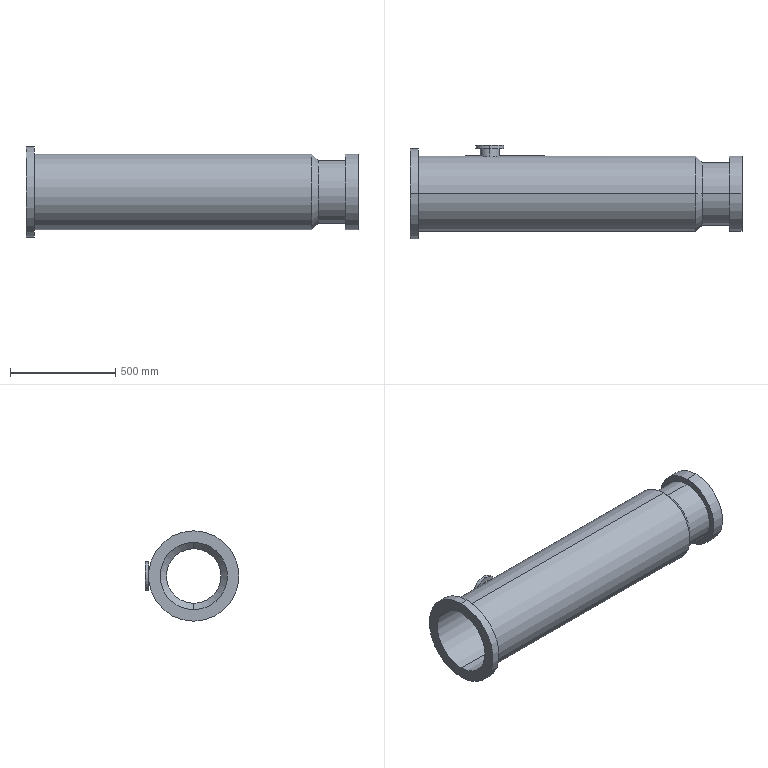Part | SolidWorks | features ICE 4, Revolution 1 | 1 solid | 28 faces | box 1580 x 445 x 430 mm | volume 36909179 mm3 | cylinder 18 | plane 6 | cone 4 | commonest cylinder face diameters 360 x4 80 x2 92 x2 135 x2 260 x2 300 x2
STEP:
#1=CARTESIAN_POINT('',(380.,230.,67.5));
#2=VERTEX_POINT('',#1);
#3=CARTESIAN_POINT('',(380.,230.,-67.5));
#4=VERTEX_POINT('',#3);
#5=CARTESIAN_POINT('',(380.,230.,0.));
#6=DIRECTION('',(0.,1.,0.));
#7=DIRECTION('',(0.,0.,1.));
#8=AXIS2_PLACEMENT_3D('',#5,#6,#7);
#9=CIRCLE('',#8,67.5);
#10=EDGE_CURVE('',#2,#4,#9,.T.);
#11=ORIENTED_EDGE('',*,*,#10,.F.);
#12=CARTESIAN_POINT('',(380.,215.,67.5));
#13=VERTEX_POINT('',#12);
#14=CARTESIAN_POINT('',(380.,230.,67.5));
#15=DIRECTION('',(0.,-1.,0.));
#16=VECTOR('',#15,1000.);
#17=LINE('',#14,#16);
#18=EDGE_CURVE('',#2,#13,#17,.T.);
#19=ORIENTED_EDGE('',*,*,#18,.T.);
#20=CARTESIAN_POINT('',(380.,215.,-67.5));
#21=VERTEX_POINT('',#20);
#22=CARTESIAN_POINT('',(380.,215.,0.));
#23=DIRECTION('',(0.,1.,0.));
#24=DIRECTION('',(0.,0.,1.));
#25=AXIS2_PLACEMENT_3D('',#22,#23,#24);
#26=CIRCLE('',#25,67.5);
#27=EDGE_CURVE('',#13,#21,#26,.T.);
#28=ORIENTED_EDGE('',*,*,#27,.T.);
#29=CARTESIAN_POINT('',(380.,230.,-67.5));
#30=DIRECTION('',(0.,-1.,0.));
#31=VECTOR('',#30,1000.);
#32=LINE('',#29,#31);
#33=EDGE_CURVE('',#4,#21,#32,.T.);
#34=ORIENTED_EDGE('',*,*,#33,.F.);
#35=EDGE_LOOP('',(#11,#19,#28,#34));
#36=FACE_OUTER_BOUND('',#35,.T.);
#37=CARTESIAN_POINT('',(380.,230.,0.));
#38=DIRECTION('',(0.,-1.,0.));
#39=DIRECTION('',(0.,0.,-1.));
#40=AXIS2_PLACEMENT_3D('',#37,#38,#39);
#41=CYLINDRICAL_SURFACE('',#40,67.5);
#42=ADVANCED_FACE('',(#36),#41,.T.);
#43=CARTESIAN_POINT('',(1351.716,0.,-160.));
#44=VERTEX_POINT('',#43);
#45=CARTESIAN_POINT('',(1351.716,0.,160.));
#46=VERTEX_POINT('',#45);
#47=CARTESIAN_POINT('',(1351.716,0.,0.));
#48=DIRECTION('',(-1.,0.,0.));
#49=DIRECTION('',(0.,0.,1.));
#50=AXIS2_PLACEMENT_3D('',#47,#48,#49);
#51=CIRCLE('',#50,160.);
#52=EDGE_CURVE('',#44,#46,#51,.T.);
#53=ORIENTED_EDGE('',*,*,#52,.F.);
#54=CARTESIAN_POINT('',(0.,0.,-160.));
#55=VERTEX_POINT('',#54);
#56=CARTESIAN_POINT('',(0.,0.,-160.));
#57=DIRECTION('',(-1.,0.,0.));
#58=VECTOR('',#57,1000.);
#59=LINE('',#56,#58);
#60=EDGE_CURVE('',#44,#55,#59,.T.);
#61=ORIENTED_EDGE('',*,*,#60,.T.);
#62=CARTESIAN_POINT('',(0.,0.,160.));
#63=VERTEX_POINT('',#62);
#64=CARTESIAN_POINT('',(0.,0.,0.));
#65=DIRECTION('',(-1.,0.,0.));
#66=DIRECTION('',(0.,0.,1.));
#67=AXIS2_PLACEMENT_3D('',#64,#65,#66);
#68=CIRCLE('',#67,160.);
#69=EDGE_CURVE('',#55,#63,#68,.T.);
#70=ORIENTED_EDGE('',*,*,#69,.T.);
#71=CARTESIAN_POINT('',(0.,0.,160.));
#72=DIRECTION('',(-1.,0.,0.));
#73=VECTOR('',#72,1000.);
#74=LINE('',#71,#73);
#75=EDGE_CURVE('',#46,#63,#74,.T.);
#76=ORIENTED_EDGE('',*,*,#75,.F.);
#77=EDGE_LOOP('',(#53,#61,#70,#76));
#78=FACE_OUTER_BOUND('',#77,.T.);
#79=CARTESIAN_POINT('',(0.,0.,0.));
#80=DIRECTION('',(-1.,0.,0.));
#81=DIRECTION('',(0.,0.,1.));
#82=AXIS2_PLACEMENT_3D('',#79,#80,#81);
#83=CYLINDRICAL_SURFACE('',#82,160.);
#84=ADVANCED_FACE('',(#78),#83,.F.);
#85=CARTESIAN_POINT('',(380.,230.,-40.));
#86=VERTEX_POINT('',#85);
#87=CARTESIAN_POINT('',(380.,230.,40.));
#88=VERTEX_POINT('',#87);
#89=CARTESIAN_POINT('',(380.,230.,0.));
#90=DIRECTION('',(0.,1.,0.));
#91=DIRECTION('',(0.,0.,1.));
#92=AXIS2_PLACEMENT_3D('',#89,#90,#91);
#93=CIRCLE('',#92,40.);
#94=EDGE_CURVE('',#86,#88,#93,.T.);
#95=ORIENTED_EDGE('',*,*,#94,.T.);
#96=CARTESIAN_POINT('',(380.,154.919,40.));
#97=VERTEX_POINT('',#96);
#98=CARTESIAN_POINT('',(380.,215.,40.));
#99=DIRECTION('',(0.,-1.,0.));
#100=VECTOR('',#99,1000.);
#101=LINE('',#98,#100);
#102=EDGE_CURVE('',#88,#97,#101,.T.);
#103=ORIENTED_EDGE('',*,*,#102,.T.);
#104=CARTESIAN_POINT('',(380.,154.919,-40.));
#105=VERTEX_POINT('',#104);
#106=CARTESIAN_POINT('',(380.,154.919,-40.));
#107=CARTESIAN_POINT('',(377.384,154.919,-40.));
#108=CARTESIAN_POINT('',(374.776,154.986,-39.746));
#109=CARTESIAN_POINT('',(369.578,155.248,-38.709));
#110=CARTESIAN_POINT('',(367.077,155.439,-37.945));
#111=CARTESIAN_POINT('',(363.464,155.795,-36.445));
#112=CARTESIAN_POINT('',(362.283,155.925,-35.886));
#113=CARTESIAN_POINT('',(360.547,156.135,-34.957));
#114=CARTESIAN_POINT('',(359.973,156.207,-34.632));
#115=CARTESIAN_POINT('',(358.846,156.356,-33.955));
#116=CARTESIAN_POINT('',(358.293,156.432,-33.604));
#117=CARTESIAN_POINT('',(355.581,156.817,-31.789));
#118=CARTESIAN_POINT('',(353.574,157.147,-30.141));
#119=CARTESIAN_POINT('',(351.268,157.561,-27.837));
#120=CARTESIAN_POINT('',(350.817,157.643,-27.364));
#121=CARTESIAN_POINT('',(349.936,157.809,-26.392));
#122=CARTESIAN_POINT('',(349.505,157.892,-25.894));
#123=CARTESIAN_POINT('',(348.257,158.136,-24.375));
#124=CARTESIAN_POINT('',(347.481,158.294,-23.328));
#125=CARTESIAN_POINT('',(345.312,158.749,-20.088));
#126=CARTESIAN_POINT('',(344.079,159.026,-17.795));
#127=CARTESIAN_POINT('',(342.814,159.32,-14.753));
#128=CARTESIAN_POINT('',(342.575,159.376,-14.136));
#129=CARTESIAN_POINT('',(342.131,159.48,-12.898));
#130=CARTESIAN_POINT('',(341.924,159.53,-12.275));
#131=CARTESIAN_POINT('',(341.353,159.667,-10.397));
#132=CARTESIAN_POINT('',(341.034,159.744,-9.131));
#133=CARTESIAN_POINT('',(340.522,159.87,-6.571));
#134=CARTESIAN_POINT('',(340.328,159.918,-5.277));
#135=CARTESIAN_POINT('',(340.132,159.967,-3.315));
#136=CARTESIAN_POINT('',(340.083,159.979,-2.658));
#137=CARTESIAN_POINT('',(340.017,159.996,-1.335));
#138=CARTESIAN_POINT('',(340.,160.,-0.6716));
#139=CARTESIAN_POINT('',(339.999,160.,2.626));
#140=CARTESIAN_POINT('',(340.257,159.935,5.229));
#141=CARTESIAN_POINT('',(341.023,159.747,9.083));
#142=CARTESIAN_POINT('',(341.342,159.669,10.36));
#143=CARTESIAN_POINT('',(342.111,159.485,12.891));
#144=CARTESIAN_POINT('',(342.555,159.38,14.127));
#145=CARTESIAN_POINT('',(344.057,159.031,17.745));
#146=CARTESIAN_POINT('',(345.284,158.755,20.042));
#147=CARTESIAN_POINT('',(347.106,158.373,22.768));
#148=CARTESIAN_POINT('',(347.486,158.294,23.308));
#149=CARTESIAN_POINT('',(348.268,158.135,24.362));
#150=CARTESIAN_POINT('',(348.671,158.055,24.878));
#151=CARTESIAN_POINT('',(349.912,157.812,26.39));
#152=CARTESIAN_POINT('',(350.785,157.647,27.352));
#153=CARTESIAN_POINT('',(352.619,157.318,29.189));
#154=CARTESIAN_POINT('',(353.581,157.153,30.062));
#155=CARTESIAN_POINT('',(355.092,156.908,31.305));
#156=CARTESIAN_POINT('',(355.607,156.827,31.708));
#157=CARTESIAN_POINT('',(356.66,156.667,32.491));
#158=CARTESIAN_POINT('',(357.198,156.587,32.871));
#159=CARTESIAN_POINT('',(359.922,156.2,34.695));
#160=CARTESIAN_POINT('',(362.216,155.918,35.924));
#161=CARTESIAN_POINT('',(365.826,155.562,37.427));
#162=CARTESIAN_POINT('',(367.058,155.454,37.871));
#163=CARTESIAN_POINT('',(368.95,155.312,38.449));
#164=CARTESIAN_POINT('',(369.589,155.267,38.627));
#165=CARTESIAN_POINT('',(370.868,155.187,38.949));
#166=CARTESIAN_POINT('',(371.51,155.15,39.094));
#167=CARTESIAN_POINT('',(374.731,154.988,39.739));
#168=CARTESIAN_POINT('',(377.346,154.919,40.));
#169=CARTESIAN_POINT('',(380.,154.919,40.));
#170=B_SPLINE_CURVE_WITH_KNOTS('',3,(#106,#107,#108,#109,#110,#111,#112,#113,#114,#115,#116,#117,#118,#119,#120,#121,#122,#123,#124,#125,#126,#127,#128,#129,#130,#131,#132,#133,#134,#135,#136,#137,#138,#139,#140,#141,#142,#143,#144,#145,#146,#147,#148,#149,#150,#151,#152,#153,#154,#155,#156,#157,#158,#159,#160,#161,#162,#163,#164,#165,#166,#167,#168,#169),.UNSPECIFIED.,.F.,.F.,(4,2,2,2,2,2,2,2,2,2,2,2,2,2,2,2,2,2,2,2,2,2,2,2,2,2,2,2,2,2,2,4),(0.1256,0.1334,0.1412,0.1452,0.1471,0.1491,0.1569,0.1589,0.1609,0.1648,0.1726,0.1746,0.1766,0.1805,0.1844,0.1864,0.1883,0.1962,0.2001,0.204,0.2119,0.2138,0.2158,0.2197,0.2236,0.2256,0.2275,0.2354,0.2393,0.2413,0.2432,0.2511),.UNSPECIFIED.);
#171=EDGE_CURVE('',#105,#97,#170,.T.);
#172=ORIENTED_EDGE('',*,*,#171,.F.);
#173=CARTESIAN_POINT('',(380.,215.,-40.));
#174=DIRECTION('',(0.,-1.,0.));
#175=VECTOR('',#174,1000.);
#176=LINE('',#173,#175);
#177=EDGE_CURVE('',#86,#105,#176,.T.);
#178=ORIENTED_EDGE('',*,*,#177,.F.);
#179=EDGE_LOOP('',(#95,#103,#172,#178));
#180=FACE_OUTER_BOUND('',#179,.T.);
#181=CARTESIAN_POINT('',(380.,215.,0.));
#182=DIRECTION('',(0.,-1.,0.));
#183=DIRECTION('',(0.,0.,-1.));
#184=AXIS2_PLACEMENT_3D('',#181,#182,#183);
#185=CYLINDRICAL_SURFACE('',#184,40.);
#186=ADVANCED_FACE('',(#180),#185,.F.);
#187=CARTESIAN_POINT('',(380.,215.,46.));
#188=VERTEX_POINT('',#187);
#189=CARTESIAN_POINT('',(380.,215.,-46.));
#190=VERTEX_POINT('',#189);
#191=CARTESIAN_POINT('',(380.,215.,0.));
#192=DIRECTION('',(0.,1.,0.));
#193=DIRECTION('',(0.,0.,1.));
#194=AXIS2_PLACEMENT_3D('',#191,#192,#193);
#195=CIRCLE('',#194,46.);
#196=EDGE_CURVE('',#188,#190,#195,.T.);
#197=ORIENTED_EDGE('',*,*,#196,.F.);
#198=CARTESIAN_POINT('',(380.,174.023,46.));
#199=VERTEX_POINT('',#198);
#200=CARTESIAN_POINT('',(380.,215.,46.));
#201=DIRECTION('',(0.,-1.,0.));
#202=VECTOR('',#201,1000.);
#203=LINE('',#200,#202);
#204=EDGE_CURVE('',#188,#199,#203,.T.);
#205=ORIENTED_EDGE('',*,*,#204,.T.);
#206=CARTESIAN_POINT('',(380.,174.023,-46.));
#207=VERTEX_POINT('',#206);
#208=CARTESIAN_POINT('',(380.,174.023,46.));
#209=CARTESIAN_POINT('',(383.009,174.023,46.));
#210=CARTESIAN_POINT('',(386.01,174.101,45.707));
#211=CARTESIAN_POINT('',(391.987,174.41,44.515));
#212=CARTESIAN_POINT('',(394.863,174.635,43.636));
#213=CARTESIAN_POINT('',(399.018,175.054,41.911));
#214=CARTESIAN_POINT('',(400.377,175.207,41.268));
#215=CARTESIAN_POINT('',(402.374,175.454,40.199));
#216=CARTESIAN_POINT('',(403.034,175.54,39.825));
#217=CARTESIAN_POINT('',(404.329,175.714,39.047));
#218=CARTESIAN_POINT('',(404.965,175.803,38.644));
#219=CARTESIAN_POINT('',(408.083,176.257,36.556));
#220=CARTESIAN_POINT('',(410.39,176.644,34.662));
#221=CARTESIAN_POINT('',(413.042,177.131,32.012));
#222=CARTESIAN_POINT('',(413.561,177.229,31.468));
#223=CARTESIAN_POINT('',(414.575,177.424,30.35));
#224=CARTESIAN_POINT('',(415.07,177.521,29.777));
#225=CARTESIAN_POINT('',(416.504,177.808,28.031));
#226=CARTESIAN_POINT('',(417.396,177.994,26.828));
#227=CARTESIAN_POINT('',(419.89,178.529,23.103));
#228=CARTESIAN_POINT('',(421.308,178.855,20.466));
#229=CARTESIAN_POINT('',(422.763,179.2,16.967));
#230=CARTESIAN_POINT('',(423.038,179.266,16.257));
#231=CARTESIAN_POINT('',(423.549,179.389,14.834));
#232=CARTESIAN_POINT('',(423.786,179.447,14.118));
#233=CARTESIAN_POINT('',(424.444,179.608,11.958));
#234=CARTESIAN_POINT('',(424.81,179.699,10.502));
#235=CARTESIAN_POINT('',(425.4,179.847,7.558));
#236=CARTESIAN_POINT('',(425.623,179.904,6.069));
#237=CARTESIAN_POINT('',(425.848,179.961,3.812));
#238=CARTESIAN_POINT('',(425.905,179.976,3.056));
#239=CARTESIAN_POINT('',(425.981,179.995,1.534));
#240=CARTESIAN_POINT('',(426.,180.,0.7712));
#241=CARTESIAN_POINT('',(426.001,180.,-3.021));
#242=CARTESIAN_POINT('',(425.704,179.924,-6.015));
#243=CARTESIAN_POINT('',(424.97,179.739,-9.709));
#244=CARTESIAN_POINT('',(424.805,179.698,-10.445));
#245=CARTESIAN_POINT('',(424.437,179.607,-11.913));
#246=CARTESIAN_POINT('',(424.234,179.557,-12.645));
#247=CARTESIAN_POINT('',(423.571,179.394,-14.828));
#248=CARTESIAN_POINT('',(423.061,179.271,-16.248));
#249=CARTESIAN_POINT('',(421.334,178.861,-20.409));
#250=CARTESIAN_POINT('',(419.922,178.536,-23.051));
#251=CARTESIAN_POINT('',(417.826,178.086,-26.187));
#252=CARTESIAN_POINT('',(417.389,177.994,-26.807));
#253=CARTESIAN_POINT('',(416.49,177.807,-28.019));
#254=CARTESIAN_POINT('',(416.027,177.713,-28.611));
#255=CARTESIAN_POINT('',(414.6,177.427,-30.349));
#256=CARTESIAN_POINT('',(413.597,177.233,-31.456));
#257=CARTESIAN_POINT('',(411.487,176.846,-33.567));
#258=CARTESIAN_POINT('',(410.381,176.651,-34.572));
#259=CARTESIAN_POINT('',(408.644,176.364,-36.001));
#260=CARTESIAN_POINT('',(408.052,176.268,-36.465));
#261=CARTESIAN_POINT('',(406.84,176.08,-37.365));
#262=CARTESIAN_POINT('',(406.221,175.986,-37.803));
#263=CARTESIAN_POINT('',(403.09,175.531,-39.899));
#264=CARTESIAN_POINT('',(400.453,175.199,-41.312));
#265=CARTESIAN_POINT('',(396.301,174.779,-43.041));
#266=CARTESIAN_POINT('',(394.884,174.652,-43.552));
#267=CARTESIAN_POINT('',(392.706,174.485,-44.217));
#268=CARTESIAN_POINT('',(391.972,174.433,-44.421));
#269=CARTESIAN_POINT('',(390.502,174.338,-44.792));
#270=CARTESIAN_POINT('',(389.764,174.295,-44.958));
#271=CARTESIAN_POINT('',(386.06,174.103,-45.699));
#272=CARTESIAN_POINT('',(383.052,174.023,-46.));
#273=CARTESIAN_POINT('',(380.,174.023,-46.));
#274=B_SPLINE_CURVE_WITH_KNOTS('',3,(#208,#209,#210,#211,#212,#213,#214,#215,#216,#217,#218,#219,#220,#221,#222,#223,#224,#225,#226,#227,#228,#229,#230,#231,#232,#233,#234,#235,#236,#237,#238,#239,#240,#241,#242,#243,#244,#245,#246,#247,#248,#249,#250,#251,#252,#253,#254,#255,#256,#257,#258,#259,#260,#261,#262,#263,#264,#265,#266,#267,#268,#269,#270,#271,#272,#273),.UNSPECIFIED.,.F.,.F.,(4,2,2,2,2,2,2,2,2,2,2,2,2,2,2,2,2,2,2,2,2,2,2,2,2,2,2,2,2,2,2,2,4),(0.1444,0.1534,0.1625,0.167,0.1692,0.1715,0.1805,0.1828,0.185,0.1895,0.1986,0.2008,0.2031,0.2076,0.2121,0.2143,0.2166,0.2256,0.2279,0.2301,0.2347,0.2437,0.2459,0.2482,0.2527,0.2572,0.2595,0.2617,0.2707,0.2753,0.2775,0.2798,0.2888),.UNSPECIFIED.);
#275=EDGE_CURVE('',#199,#207,#274,.T.);
#276=ORIENTED_EDGE('',*,*,#275,.T.);
#277=CARTESIAN_POINT('',(380.,215.,-46.));
#278=DIRECTION('',(0.,-1.,0.));
#279=VECTOR('',#278,1000.);
#280=LINE('',#277,#279);
#281=EDGE_CURVE('',#190,#207,#280,.T.);
#282=ORIENTED_EDGE('',*,*,#281,.F.);
#283=EDGE_LOOP('',(#197,#205,#276,#282));
#284=FACE_OUTER_BOUND('',#283,.T.);
#285=CARTESIAN_POINT('',(380.,215.,0.));
#286=DIRECTION('',(0.,-1.,0.));
#287=DIRECTION('',(0.,0.,-1.));
#288=AXIS2_PLACEMENT_3D('',#285,#286,#287);
#289=CYLINDRICAL_SURFACE('',#288,46.);
#290=ADVANCED_FACE('',(#284),#289,.T.);
#291=CARTESIAN_POINT('',(1381.716,0.,-130.));
#292=VERTEX_POINT('',#291);
#293=CARTESIAN_POINT('',(1381.716,0.,130.));
#294=VERTEX_POINT('',#293);
#295=CARTESIAN_POINT('',(1381.716,0.,0.));
#296=DIRECTION('',(-1.,0.,0.));
#297=DIRECTION('',(0.,0.,1.));
#298=AXIS2_PLACEMENT_3D('',#295,#296,#297);
#299=CIRCLE('',#298,130.);
#300=EDGE_CURVE('',#292,#294,#299,.T.);
#301=ORIENTED_EDGE('',*,*,#300,.F.);
#302=CARTESIAN_POINT('',(1351.716,0.,-160.));
#303=DIRECTION('',(-0.7071,0.,-0.7071));
#304=VECTOR('',#303,1000.);
#305=LINE('',#302,#304);
#306=EDGE_CURVE('',#292,#44,#305,.T.);
#307=ORIENTED_EDGE('',*,*,#306,.T.);
#308=ORIENTED_EDGE('',*,*,#52,.T.);
#309=CARTESIAN_POINT('',(1351.716,0.,160.));
#310=DIRECTION('',(-0.7071,0.,0.7071));
#311=VECTOR('',#310,1000.);
#312=LINE('',#309,#311);
#313=EDGE_CURVE('',#294,#46,#312,.T.);
#314=ORIENTED_EDGE('',*,*,#313,.F.);
#315=EDGE_LOOP('',(#301,#307,#308,#314));
#316=FACE_OUTER_BOUND('',#315,.T.);
#317=CARTESIAN_POINT('',(1351.716,0.,0.));
#318=DIRECTION('',(-1.,0.,0.));
#319=DIRECTION('',(0.,0.,1.));
#320=AXIS2_PLACEMENT_3D('',#317,#318,#319);
#321=CONICAL_SURFACE('',#320,160.,0.7854);
#322=ADVANCED_FACE('',(#316),#321,.F.);
#323=CARTESIAN_POINT('',(1580.,0.,-130.));
#324=VERTEX_POINT('',#323);
#325=CARTESIAN_POINT('',(1580.,0.,130.));
#326=VERTEX_POINT('',#325);
#327=CARTESIAN_POINT('',(1580.,0.,0.));
#328=DIRECTION('',(-1.,0.,0.));
#329=DIRECTION('',(0.,0.,1.));
#330=AXIS2_PLACEMENT_3D('',#327,#328,#329);
#331=CIRCLE('',#330,130.);
#332=EDGE_CURVE('',#324,#326,#331,.T.);
#333=ORIENTED_EDGE('',*,*,#332,.F.);
#334=CARTESIAN_POINT('',(0.,0.,-130.));
#335=DIRECTION('',(-1.,0.,0.));
#336=VECTOR('',#335,1000.);
#337=LINE('',#334,#336);
#338=EDGE_CURVE('',#324,#292,#337,.T.);
#339=ORIENTED_EDGE('',*,*,#338,.T.);
#340=ORIENTED_EDGE('',*,*,#300,.T.);
#341=CARTESIAN_POINT('',(0.,0.,130.));
#342=DIRECTION('',(-1.,0.,0.));
#343=VECTOR('',#342,1000.);
#344=LINE('',#341,#343);
#345=EDGE_CURVE('',#326,#294,#344,.T.);
#346=ORIENTED_EDGE('',*,*,#345,.F.);
#347=EDGE_LOOP('',(#333,#339,#340,#346));
#348=FACE_OUTER_BOUND('',#347,.T.);
#349=CARTESIAN_POINT('',(0.,0.,0.));
#350=DIRECTION('',(-1.,0.,0.));
#351=DIRECTION('',(0.,0.,1.));
#352=AXIS2_PLACEMENT_3D('',#349,#350,#351);
#353=CYLINDRICAL_SURFACE('',#352,130.);
#354=ADVANCED_FACE('',(#348),#353,.F.);
#355=CARTESIAN_POINT('',(1580.,0.,180.));
#356=VERTEX_POINT('',#355);
#357=CARTESIAN_POINT('',(1580.,0.,-180.));
#358=VERTEX_POINT('',#357);
#359=CARTESIAN_POINT('',(1580.,0.,0.));
#360=DIRECTION('',(-1.,0.,0.));
#361=DIRECTION('',(0.,0.,1.));
#362=AXIS2_PLACEMENT_3D('',#359,#360,#361);
#363=CIRCLE('',#362,180.);
#364=EDGE_CURVE('',#356,#358,#363,.T.);
#365=ORIENTED_EDGE('',*,*,#364,.T.);
#366=CARTESIAN_POINT('',(1520.,0.,-180.));
#367=VERTEX_POINT('',#366);
#368=CARTESIAN_POINT('',(0.,0.,-180.));
#369=DIRECTION('',(-1.,0.,0.));
#370=VECTOR('',#369,1000.);
#371=LINE('',#368,#370);
#372=EDGE_CURVE('',#358,#367,#371,.T.);
#373=ORIENTED_EDGE('',*,*,#372,.T.);
#374=CARTESIAN_POINT('',(1520.,0.,180.));
#375=VERTEX_POINT('',#374);
#376=CARTESIAN_POINT('',(1520.,0.,0.));
#377=DIRECTION('',(-1.,0.,0.));
#378=DIRECTION('',(0.,0.,1.));
#379=AXIS2_PLACEMENT_3D('',#376,#377,#378);
#380=CIRCLE('',#379,180.);
#381=EDGE_CURVE('',#375,#367,#380,.T.);
#382=ORIENTED_EDGE('',*,*,#381,.F.);
#383=CARTESIAN_POINT('',(0.,0.,180.));
#384=DIRECTION('',(-1.,0.,0.));
#385=VECTOR('',#384,1000.);
#386=LINE('',#383,#385);
#387=EDGE_CURVE('',#356,#375,#386,.T.);
#388=ORIENTED_EDGE('',*,*,#387,.F.);
#389=EDGE_LOOP('',(#365,#373,#382,#388));
#390=FACE_OUTER_BOUND('',#389,.T.);
#391=CARTESIAN_POINT('',(0.,0.,0.));
#392=DIRECTION('',(-1.,0.,0.));
#393=DIRECTION('',(0.,0.,1.));
#394=AXIS2_PLACEMENT_3D('',#391,#392,#393);
#395=CYLINDRICAL_SURFACE('',#394,180.);
#396=ADVANCED_FACE('',(#390),#395,.T.);
#397=CARTESIAN_POINT('',(1520.,0.,150.));
#398=VERTEX_POINT('',#397);
#399=CARTESIAN_POINT('',(1520.,0.,-150.));
#400=VERTEX_POINT('',#399);
#401=CARTESIAN_POINT('',(1520.,0.,0.));
#402=DIRECTION('',(-1.,0.,0.));
#403=DIRECTION('',(0.,0.,1.));
#404=AXIS2_PLACEMENT_3D('',#401,#402,#403);
#405=CIRCLE('',#404,150.);
#406=EDGE_CURVE('',#398,#400,#405,.T.);
#407=ORIENTED_EDGE('',*,*,#406,.T.);
#408=CARTESIAN_POINT('',(1390.,0.,-150.));
#409=VERTEX_POINT('',#408);
#410=CARTESIAN_POINT('',(0.,0.,-150.));
#411=DIRECTION('',(-1.,0.,0.));
#412=VECTOR('',#411,1000.);
#413=LINE('',#410,#412);
#414=EDGE_CURVE('',#400,#409,#413,.T.);
#415=ORIENTED_EDGE('',*,*,#414,.T.);
#416=CARTESIAN_POINT('',(1390.,0.,150.));
#417=VERTEX_POINT('',#416);
#418=CARTESIAN_POINT('',(1390.,0.,0.));
#419=DIRECTION('',(-1.,0.,0.));
#420=DIRECTION('',(0.,0.,1.));
#421=AXIS2_PLACEMENT_3D('',#418,#419,#420);
#422=CIRCLE('',#421,150.);
#423=EDGE_CURVE('',#417,#409,#422,.T.);
#424=ORIENTED_EDGE('',*,*,#423,.F.);
#425=CARTESIAN_POINT('',(0.,0.,150.));
#426=DIRECTION('',(-1.,0.,0.));
#427=VECTOR('',#426,1000.);
#428=LINE('',#425,#427);
#429=EDGE_CURVE('',#398,#417,#428,.T.);
#430=ORIENTED_EDGE('',*,*,#429,.F.);
#431=EDGE_LOOP('',(#407,#415,#424,#430));
#432=FACE_OUTER_BOUND('',#431,.T.);
#433=CARTESIAN_POINT('',(0.,0.,0.));
#434=DIRECTION('',(-1.,0.,0.));
#435=DIRECTION('',(0.,0.,1.));
#436=AXIS2_PLACEMENT_3D('',#433,#434,#435);
#437=CYLINDRICAL_SURFACE('',#436,150.);
#438=ADVANCED_FACE('',(#432),#437,.T.);
#439=ORIENTED_EDGE('',*,*,#423,.T.);
#440=CARTESIAN_POINT('',(1360.,0.,-180.));
#441=VERTEX_POINT('',#440);
#442=CARTESIAN_POINT('',(1390.,0.,-150.));
#443=DIRECTION('',(-0.7071,0.,-0.7071));
#444=VECTOR('',#443,1000.);
#445=LINE('',#442,#444);
#446=EDGE_CURVE('',#409,#441,#445,.T.);
#447=ORIENTED_EDGE('',*,*,#446,.T.);
#448=CARTESIAN_POINT('',(1360.,0.,180.));
#449=VERTEX_POINT('',#448);
#450=CARTESIAN_POINT('',(1360.,0.,0.));
#451=DIRECTION('',(-1.,0.,0.));
#452=DIRECTION('',(0.,0.,1.));
#453=AXIS2_PLACEMENT_3D('',#450,#451,#452);
#454=CIRCLE('',#453,180.);
#455=EDGE_CURVE('',#449,#441,#454,.T.);
#456=ORIENTED_EDGE('',*,*,#455,.F.);
#457=CARTESIAN_POINT('',(1390.,0.,150.));
#458=DIRECTION('',(-0.7071,0.,0.7071));
#459=VECTOR('',#458,1000.);
#460=LINE('',#457,#459);
#461=EDGE_CURVE('',#417,#449,#460,.T.);
#462=ORIENTED_EDGE('',*,*,#461,.F.);
#463=EDGE_LOOP('',(#439,#447,#456,#462));
#464=FACE_OUTER_BOUND('',#463,.T.);
#465=CARTESIAN_POINT('',(1390.,0.,0.));
#466=DIRECTION('',(-1.,0.,0.));
#467=DIRECTION('',(0.,0.,1.));
#468=AXIS2_PLACEMENT_3D('',#465,#466,#467);
#469=CONICAL_SURFACE('',#468,150.,0.7854);
#470=ADVANCED_FACE('',(#464),#469,.T.);
#471=CARTESIAN_POINT('',(40.,0.,215.));
#472=VERTEX_POINT('',#471);
#473=CARTESIAN_POINT('',(40.,0.,-215.));
#474=VERTEX_POINT('',#473);
#475=CARTESIAN_POINT('',(40.,0.,0.));
#476=DIRECTION('',(-1.,0.,0.));
#477=DIRECTION('',(0.,0.,1.));
#478=AXIS2_PLACEMENT_3D('',#475,#476,#477);
#479=CIRCLE('',#478,215.);
#480=EDGE_CURVE('',#472,#474,#479,.T.);
#481=ORIENTED_EDGE('',*,*,#480,.T.);
#482=CARTESIAN_POINT('',(0.,0.,-215.));
#483=VERTEX_POINT('',#482);
#484=CARTESIAN_POINT('',(0.,0.,-215.));
#485=DIRECTION('',(-1.,0.,0.));
#486=VECTOR('',#485,1000.);
#487=LINE('',#484,#486);
#488=EDGE_CURVE('',#474,#483,#487,.T.);
#489=ORIENTED_EDGE('',*,*,#488,.T.);
#490=CARTESIAN_POINT('',(0.,0.,215.));
#491=VERTEX_POINT('',#490);
#492=CARTESIAN_POINT('',(0.,0.,0.));
#493=DIRECTION('',(-1.,0.,0.));
#494=DIRECTION('',(0.,0.,1.));
#495=AXIS2_PLACEMENT_3D('',#492,#493,#494);
#496=CIRCLE('',#495,215.);
#497=EDGE_CURVE('',#491,#483,#496,.T.);
#498=ORIENTED_EDGE('',*,*,#497,.F.);
#499=CARTESIAN_POINT('',(0.,0.,215.));
#500=DIRECTION('',(-1.,0.,0.));
#501=VECTOR('',#500,1000.);
#502=LINE('',#499,#501);
#503=EDGE_CURVE('',#472,#491,#502,.T.);
#504=ORIENTED_EDGE('',*,*,#503,.F.);
#505=EDGE_LOOP('',(#481,#489,#498,#504));
#506=FACE_OUTER_BOUND('',#505,.T.);
#507=CARTESIAN_POINT('',(0.,0.,0.));
#508=DIRECTION('',(-1.,0.,0.));
#509=DIRECTION('',(0.,0.,1.));
#510=AXIS2_PLACEMENT_3D('',#507,#508,#509);
#511=CYLINDRICAL_SURFACE('',#510,215.);
#512=ADVANCED_FACE('',(#506),#511,.T.);
#513=CARTESIAN_POINT('',(380.,174.023,-46.));
#514=CARTESIAN_POINT('',(376.947,174.023,-46.));
#515=CARTESIAN_POINT('',(373.948,174.103,-45.699));
#516=CARTESIAN_POINT('',(369.525,174.332,-44.817));
#517=CARTESIAN_POINT('',(368.064,174.426,-44.45));
#518=CARTESIAN_POINT('',(365.891,174.592,-43.79));
#519=CARTESIAN_POINT('',(365.169,174.652,-43.55));
#520=CARTESIAN_POINT('',(363.74,174.779,-43.037));
#521=CARTESIAN_POINT('',(363.036,174.847,-42.764));
#522=CARTESIAN_POINT('',(359.558,175.198,-41.318));
#523=CARTESIAN_POINT('',(356.921,175.529,-39.904));
#524=CARTESIAN_POINT('',(353.802,175.983,-37.818));
#525=CARTESIAN_POINT('',(353.187,176.076,-37.385));
#526=CARTESIAN_POINT('',(351.975,176.264,-36.485));
#527=CARTESIAN_POINT('',(351.377,176.36,-36.018));
#528=CARTESIAN_POINT('',(349.631,176.649,-34.583));
#529=CARTESIAN_POINT('',(348.522,176.844,-33.576));
#530=CARTESIAN_POINT('',(345.354,177.426,-30.407));
#531=CARTESIAN_POINT('',(343.454,177.811,-28.099));
#532=CARTESIAN_POINT('',(341.352,178.262,-24.958));
#533=CARTESIAN_POINT('',(340.946,178.351,-24.318));
#534=CARTESIAN_POINT('',(340.17,178.522,-23.025));
#535=CARTESIAN_POINT('',(339.799,178.606,-22.371));
#536=CARTESIAN_POINT('',(338.737,178.847,-20.386));
#537=CARTESIAN_POINT('',(338.096,178.996,-19.033));
#538=CARTESIAN_POINT('',(336.947,179.269,-16.268));
#539=CARTESIAN_POINT('',(336.439,179.392,-14.855));
#540=CARTESIAN_POINT('',(335.779,179.554,-12.69));
#541=CARTESIAN_POINT('',(335.576,179.604,-11.961));
#542=CARTESIAN_POINT('',(335.205,179.696,-10.486));
#543=CARTESIAN_POINT('',(335.037,179.738,-9.743));
#544=CARTESIAN_POINT('',(334.296,179.924,-6.027));
#545=CARTESIAN_POINT('',(334.001,180.,-3.034));
#546=CARTESIAN_POINT('',(333.999,180.,1.488));
#547=CARTESIAN_POINT('',(334.073,179.981,3.001));
#548=CARTESIAN_POINT('',(334.372,179.905,6.037));
#549=CARTESIAN_POINT('',(334.597,179.848,7.536));
#550=CARTESIAN_POINT('',(335.482,179.626,11.969));
#551=CARTESIAN_POINT('',(336.356,179.409,14.843));
#552=CARTESIAN_POINT('',(337.805,179.065,18.334));
#553=CARTESIAN_POINT('',(338.114,178.993,19.029));
#554=CARTESIAN_POINT('',(338.763,178.842,20.398));
#555=CARTESIAN_POINT('',(339.103,178.764,21.072));
#556=CARTESIAN_POINT('',(340.169,178.522,23.06));
#557=CARTESIAN_POINT('',(340.941,178.351,24.344));
#558=CARTESIAN_POINT('',(342.604,177.994,26.829));
#559=CARTESIAN_POINT('',(343.495,177.808,28.03));
#560=CARTESIAN_POINT('',(344.923,177.522,29.769));
#561=CARTESIAN_POINT('',(345.415,177.426,30.338));
#562=CARTESIAN_POINT('',(346.428,177.231,31.456));
#563=CARTESIAN_POINT('',(346.951,177.133,32.005));
#564=CARTESIAN_POINT('',(349.614,176.643,34.667));
#565=CARTESIAN_POINT('',(351.924,176.256,36.56));
#566=CARTESIAN_POINT('',(355.653,175.714,39.057));
#567=CARTESIAN_POINT('',(356.94,175.539,39.831));
#568=CARTESIAN_POINT('',(358.942,175.291,40.904));
#569=CARTESIAN_POINT('',(359.62,175.211,41.246));
#570=CARTESIAN_POINT('',(360.984,175.058,41.892));
#571=CARTESIAN_POINT('',(361.672,174.984,42.198));
#572=CARTESIAN_POINT('',(365.142,174.634,43.638));
#573=CARTESIAN_POINT('',(368.01,174.41,44.513));
#574=CARTESIAN_POINT('',(371.714,174.219,45.254));
#575=CARTESIAN_POINT('',(372.461,174.185,45.384));
#576=CARTESIAN_POINT('',(373.966,174.126,45.609));
#577=CARTESIAN_POINT('',(374.724,174.101,45.703));
#578=CARTESIAN_POINT('',(376.988,174.043,45.926));
#579=CARTESIAN_POINT('',(378.495,174.023,46.));
#580=CARTESIAN_POINT('',(380.,174.023,46.));
#581=B_SPLINE_CURVE_WITH_KNOTS('',3,(#513,#514,#515,#516,#517,#518,#519,#520,#521,#522,#523,#524,#525,#526,#527,#528,#529,#530,#531,#532,#533,#534,#535,#536,#537,#538,#539,#540,#541,#542,#543,#544,#545,#546,#547,#548,#549,#550,#551,#552,#553,#554,#555,#556,#557,#558,#559,#560,#561,#562,#563,#564,#565,#566,#567,#568,#569,#570,#571,#572,#573,#574,#575,#576,#577,#578,#579,#580),.UNSPECIFIED.,.F.,.F.,(4,2,2,2,2,2,2,2,2,2,2,2,2,2,2,2,2,2,2,2,2,2,2,2,2,2,2,2,2,2,2,2,2,4),(0.,0.009026,0.01354,0.0158,0.01805,0.02708,0.02933,0.03159,0.0361,0.04513,0.04739,0.04964,0.05416,0.05867,0.06093,0.06318,0.07221,0.07672,0.08123,0.09026,0.09252,0.09477,0.09929,0.1038,0.1061,0.1083,0.1173,0.1219,0.1241,0.1264,0.1354,0.1376,0.1399,0.1444),.UNSPECIFIED.);
#582=EDGE_CURVE('',#207,#199,#581,.T.);
#583=ORIENTED_EDGE('',*,*,#582,.F.);
#584=ORIENTED_EDGE('',*,*,#275,.F.);
#585=EDGE_LOOP('',(#583,#584));
#586=FACE_BOUND('',#585,.T.);
#587=ORIENTED_EDGE('',*,*,#455,.T.);
#588=CARTESIAN_POINT('',(40.,0.,-180.));
#589=VERTEX_POINT('',#588);
#590=CARTESIAN_POINT('',(0.,0.,-180.));
#591=DIRECTION('',(-1.,0.,0.));
#592=VECTOR('',#591,1000.);
#593=LINE('',#590,#592);
#594=EDGE_CURVE('',#441,#589,#593,.T.);
#595=ORIENTED_EDGE('',*,*,#594,.T.);
#596=CARTESIAN_POINT('',(40.,0.,180.));
#597=VERTEX_POINT('',#596);
#598=CARTESIAN_POINT('',(40.,0.,0.));
#599=DIRECTION('',(-1.,0.,0.));
#600=DIRECTION('',(0.,0.,1.));
#601=AXIS2_PLACEMENT_3D('',#598,#599,#600);
#602=CIRCLE('',#601,180.);
#603=EDGE_CURVE('',#597,#589,#602,.T.);
#604=ORIENTED_EDGE('',*,*,#603,.F.);
#605=CARTESIAN_POINT('',(0.,0.,180.));
#606=DIRECTION('',(-1.,0.,0.));
#607=VECTOR('',#606,1000.);
#608=LINE('',#605,#607);
#609=EDGE_CURVE('',#449,#597,#608,.T.);
#610=ORIENTED_EDGE('',*,*,#609,.F.);
#611=EDGE_LOOP('',(#587,#595,#604,#610));
#612=FACE_OUTER_BOUND('',#611,.T.);
#613=CARTESIAN_POINT('',(0.,0.,0.));
#614=DIRECTION('',(-1.,0.,0.));
#615=DIRECTION('',(0.,0.,1.));
#616=AXIS2_PLACEMENT_3D('',#613,#614,#615);
#617=CYLINDRICAL_SURFACE('',#616,180.);
#618=ADVANCED_FACE('',(#586,#612),#617,.T.);
#619=ORIENTED_EDGE('',*,*,#594,.F.);
#620=CARTESIAN_POINT('',(1360.,0.,0.));
#621=DIRECTION('',(-1.,0.,0.));
#622=DIRECTION('',(0.,0.,1.));
#623=AXIS2_PLACEMENT_3D('',#620,#621,#622);
#624=CIRCLE('',#623,180.);
#625=EDGE_CURVE('',#441,#449,#624,.T.);
#626=ORIENTED_EDGE('',*,*,#625,.T.);
#627=ORIENTED_EDGE('',*,*,#609,.T.);
#628=CARTESIAN_POINT('',(40.,0.,0.));
#629=DIRECTION('',(-1.,0.,0.));
#630=DIRECTION('',(0.,0.,1.));
#631=AXIS2_PLACEMENT_3D('',#628,#629,#630);
#632=CIRCLE('',#631,180.);
#633=EDGE_CURVE('',#589,#597,#632,.T.);
#634=ORIENTED_EDGE('',*,*,#633,.F.);
#635=EDGE_LOOP('',(#619,#626,#627,#634));
#636=FACE_OUTER_BOUND('',#635,.T.);
#637=CARTESIAN_POINT('',(0.,0.,0.));
#638=DIRECTION('',(-1.,0.,0.));
#639=DIRECTION('',(0.,0.,1.));
#640=AXIS2_PLACEMENT_3D('',#637,#638,#639);
#641=CYLINDRICAL_SURFACE('',#640,180.);
#642=ADVANCED_FACE('',(#636),#641,.T.);
#643=ORIENTED_EDGE('',*,*,#488,.F.);
#644=CARTESIAN_POINT('',(40.,0.,0.));
#645=DIRECTION('',(-1.,0.,0.));
#646=DIRECTION('',(0.,0.,1.));
#647=AXIS2_PLACEMENT_3D('',#644,#645,#646);
#648=CIRCLE('',#647,215.);
#649=EDGE_CURVE('',#474,#472,#648,.T.);
#650=ORIENTED_EDGE('',*,*,#649,.T.);
#651=ORIENTED_EDGE('',*,*,#503,.T.);
#652=CARTESIAN_POINT('',(0.,0.,0.));
#653=DIRECTION('',(-1.,0.,0.));
#654=DIRECTION('',(0.,0.,1.));
#655=AXIS2_PLACEMENT_3D('',#652,#653,#654);
#656=CIRCLE('',#655,215.);
#657=EDGE_CURVE('',#483,#491,#656,.T.);
#658=ORIENTED_EDGE('',*,*,#657,.F.);
#659=EDGE_LOOP('',(#643,#650,#651,#658));
#660=FACE_OUTER_BOUND('',#659,.T.);
#661=CARTESIAN_POINT('',(0.,0.,0.));
#662=DIRECTION('',(-1.,0.,0.));
#663=DIRECTION('',(0.,0.,1.));
#664=AXIS2_PLACEMENT_3D('',#661,#662,#663);
#665=CYLINDRICAL_SURFACE('',#664,215.);
#666=ADVANCED_FACE('',(#660),#665,.T.);
#667=ORIENTED_EDGE('',*,*,#480,.F.);
#668=ORIENTED_EDGE('',*,*,#649,.F.);
#669=EDGE_LOOP('',(#667,#668));
#670=FACE_OUTER_BOUND('',#669,.T.);
#671=ORIENTED_EDGE('',*,*,#603,.T.);
#672=ORIENTED_EDGE('',*,*,#633,.T.);
#673=EDGE_LOOP('',(#671,#672));
#674=FACE_BOUND('',#673,.T.);
#675=CARTESIAN_POINT('',(40.,215.,0.));
#676=DIRECTION('',(-1.,0.,0.));
#677=DIRECTION('',(0.,0.,1.));
#678=AXIS2_PLACEMENT_3D('',#675,#676,#677);
#679=PLANE('',#678);
#680=ADVANCED_FACE('',(#670,#674),#679,.F.);
#681=ORIENTED_EDGE('',*,*,#446,.F.);
#682=CARTESIAN_POINT('',(1390.,0.,0.));
#683=DIRECTION('',(-1.,0.,0.));
#684=DIRECTION('',(0.,0.,1.));
#685=AXIS2_PLACEMENT_3D('',#682,#683,#684);
#686=CIRCLE('',#685,150.);
#687=EDGE_CURVE('',#409,#417,#686,.T.);
#688=ORIENTED_EDGE('',*,*,#687,.T.);
#689=ORIENTED_EDGE('',*,*,#461,.T.);
#690=ORIENTED_EDGE('',*,*,#625,.F.);
#691=EDGE_LOOP('',(#681,#688,#689,#690));
#692=FACE_OUTER_BOUND('',#691,.T.);
#693=CARTESIAN_POINT('',(1390.,0.,0.));
#694=DIRECTION('',(-1.,0.,0.));
#695=DIRECTION('',(0.,0.,1.));
#696=AXIS2_PLACEMENT_3D('',#693,#694,#695);
#697=CONICAL_SURFACE('',#696,150.,0.7854);
#698=ADVANCED_FACE('',(#692),#697,.T.);
#699=ORIENTED_EDGE('',*,*,#414,.F.);
#700=CARTESIAN_POINT('',(1520.,0.,0.));
#701=DIRECTION('',(-1.,0.,0.));
#702=DIRECTION('',(0.,0.,1.));
#703=AXIS2_PLACEMENT_3D('',#700,#701,#702);
#704=CIRCLE('',#703,150.);
#705=EDGE_CURVE('',#400,#398,#704,.T.);
#706=ORIENTED_EDGE('',*,*,#705,.T.);
#707=ORIENTED_EDGE('',*,*,#429,.T.);
#708=ORIENTED_EDGE('',*,*,#687,.F.);
#709=EDGE_LOOP('',(#699,#706,#707,#708));
#710=FACE_OUTER_BOUND('',#709,.T.);
#711=CARTESIAN_POINT('',(0.,0.,0.));
#712=DIRECTION('',(-1.,0.,0.));
#713=DIRECTION('',(0.,0.,1.));
#714=AXIS2_PLACEMENT_3D('',#711,#712,#713);
#715=CYLINDRICAL_SURFACE('',#714,150.);
#716=ADVANCED_FACE('',(#710),#715,.T.);
#717=ORIENTED_EDGE('',*,*,#406,.F.);
#718=ORIENTED_EDGE('',*,*,#705,.F.);
#719=EDGE_LOOP('',(#717,#718));
#720=FACE_BOUND('',#719,.T.);
#721=ORIENTED_EDGE('',*,*,#381,.T.);
#722=CARTESIAN_POINT('',(1520.,0.,0.));
#723=DIRECTION('',(-1.,0.,0.));
#724=DIRECTION('',(0.,0.,1.));
#725=AXIS2_PLACEMENT_3D('',#722,#723,#724);
#726=CIRCLE('',#725,180.);
#727=EDGE_CURVE('',#367,#375,#726,.T.);
#728=ORIENTED_EDGE('',*,*,#727,.T.);
#729=EDGE_LOOP('',(#721,#728));
#730=FACE_OUTER_BOUND('',#729,.T.);
#731=CARTESIAN_POINT('',(1520.,150.,0.));
#732=DIRECTION('',(1.,0.,0.));
#733=DIRECTION('',(0.,0.,-1.));
#734=AXIS2_PLACEMENT_3D('',#731,#732,#733);
#735=PLANE('',#734);
#736=ADVANCED_FACE('',(#720,#730),#735,.F.);
#737=ORIENTED_EDGE('',*,*,#372,.F.);
#738=CARTESIAN_POINT('',(1580.,0.,0.));
#739=DIRECTION('',(-1.,0.,0.));
#740=DIRECTION('',(0.,0.,1.));
#741=AXIS2_PLACEMENT_3D('',#738,#739,#740);
#742=CIRCLE('',#741,180.);
#743=EDGE_CURVE('',#358,#356,#742,.T.);
#744=ORIENTED_EDGE('',*,*,#743,.T.);
#745=ORIENTED_EDGE('',*,*,#387,.T.);
#746=ORIENTED_EDGE('',*,*,#727,.F.);
#747=EDGE_LOOP('',(#737,#744,#745,#746));
#748=FACE_OUTER_BOUND('',#747,.T.);
#749=CARTESIAN_POINT('',(0.,0.,0.));
#750=DIRECTION('',(-1.,0.,0.));
#751=DIRECTION('',(0.,0.,1.));
#752=AXIS2_PLACEMENT_3D('',#749,#750,#751);
#753=CYLINDRICAL_SURFACE('',#752,180.);
#754=ADVANCED_FACE('',(#748),#753,.T.);
#755=ORIENTED_EDGE('',*,*,#364,.F.);
#756=ORIENTED_EDGE('',*,*,#743,.F.);
#757=EDGE_LOOP('',(#755,#756));
#758=FACE_OUTER_BOUND('',#757,.T.);
#759=CARTESIAN_POINT('',(1580.,0.,0.));
#760=DIRECTION('',(-1.,0.,0.));
#761=DIRECTION('',(0.,0.,1.));
#762=AXIS2_PLACEMENT_3D('',#759,#760,#761);
#763=CIRCLE('',#762,130.);
#764=EDGE_CURVE('',#326,#324,#763,.T.);
#765=ORIENTED_EDGE('',*,*,#764,.T.);
#766=ORIENTED_EDGE('',*,*,#332,.T.);
#767=EDGE_LOOP('',(#765,#766));
#768=FACE_BOUND('',#767,.T.);
#769=CARTESIAN_POINT('',(1580.,180.,0.));
#770=DIRECTION('',(-1.,0.,0.));
#771=DIRECTION('',(0.,0.,1.));
#772=AXIS2_PLACEMENT_3D('',#769,#770,#771);
#773=PLANE('',#772);
#774=ADVANCED_FACE('',(#758,#768),#773,.F.);
#775=ORIENTED_EDGE('',*,*,#338,.F.);
#776=ORIENTED_EDGE('',*,*,#764,.F.);
#777=ORIENTED_EDGE('',*,*,#345,.T.);
#778=CARTESIAN_POINT('',(1381.716,0.,0.));
#779=DIRECTION('',(-1.,0.,0.));
#780=DIRECTION('',(0.,0.,1.));
#781=AXIS2_PLACEMENT_3D('',#778,#779,#780);
#782=CIRCLE('',#781,130.);
#783=EDGE_CURVE('',#294,#292,#782,.T.);
#784=ORIENTED_EDGE('',*,*,#783,.T.);
#785=EDGE_LOOP('',(#775,#776,#777,#784));
#786=FACE_OUTER_BOUND('',#785,.T.);
#787=CARTESIAN_POINT('',(0.,0.,0.));
#788=DIRECTION('',(-1.,0.,0.));
#789=DIRECTION('',(0.,0.,1.));
#790=AXIS2_PLACEMENT_3D('',#787,#788,#789);
#791=CYLINDRICAL_SURFACE('',#790,130.);
#792=ADVANCED_FACE('',(#786),#791,.F.);
#793=ORIENTED_EDGE('',*,*,#306,.F.);
#794=ORIENTED_EDGE('',*,*,#783,.F.);
#795=ORIENTED_EDGE('',*,*,#313,.T.);
#796=CARTESIAN_POINT('',(1351.716,0.,0.));
#797=DIRECTION('',(-1.,0.,0.));
#798=DIRECTION('',(0.,0.,1.));
#799=AXIS2_PLACEMENT_3D('',#796,#797,#798);
#800=CIRCLE('',#799,160.);
#801=EDGE_CURVE('',#46,#44,#800,.T.);
#802=ORIENTED_EDGE('',*,*,#801,.T.);
#803=EDGE_LOOP('',(#793,#794,#795,#802));
#804=FACE_OUTER_BOUND('',#803,.T.);
#805=CARTESIAN_POINT('',(1351.716,0.,0.));
#806=DIRECTION('',(-1.,0.,0.));
#807=DIRECTION('',(0.,0.,1.));
#808=AXIS2_PLACEMENT_3D('',#805,#806,#807);
#809=CONICAL_SURFACE('',#808,160.,0.7854);
#810=ADVANCED_FACE('',(#804),#809,.F.);
#811=CARTESIAN_POINT('',(0.,0.,0.));
#812=DIRECTION('',(-1.,0.,0.));
#813=DIRECTION('',(0.,0.,1.));
#814=AXIS2_PLACEMENT_3D('',#811,#812,#813);
#815=CIRCLE('',#814,160.);
#816=EDGE_CURVE('',#63,#55,#815,.T.);
#817=ORIENTED_EDGE('',*,*,#816,.F.);
#818=ORIENTED_EDGE('',*,*,#69,.F.);
#819=EDGE_LOOP('',(#817,#818));
#820=FACE_BOUND('',#819,.T.);
#821=ORIENTED_EDGE('',*,*,#497,.T.);
#822=ORIENTED_EDGE('',*,*,#657,.T.);
#823=EDGE_LOOP('',(#821,#822));
#824=FACE_OUTER_BOUND('',#823,.T.);
#825=CARTESIAN_POINT('',(0.,160.,0.));
#826=DIRECTION('',(1.,0.,0.));
#827=DIRECTION('',(0.,0.,-1.));
#828=AXIS2_PLACEMENT_3D('',#825,#826,#827);
#829=PLANE('',#828);
#830=ADVANCED_FACE('',(#820,#824),#829,.F.);
#831=ORIENTED_EDGE('',*,*,#204,.F.);
#832=CARTESIAN_POINT('',(380.,215.,0.));
#833=DIRECTION('',(0.,1.,0.));
#834=DIRECTION('',(0.,0.,1.));
#835=AXIS2_PLACEMENT_3D('',#832,#833,#834);
#836=CIRCLE('',#835,46.);
#837=EDGE_CURVE('',#190,#188,#836,.T.);
#838=ORIENTED_EDGE('',*,*,#837,.F.);
#839=ORIENTED_EDGE('',*,*,#281,.T.);
#840=ORIENTED_EDGE('',*,*,#582,.T.);
#841=EDGE_LOOP('',(#831,#838,#839,#840));
#842=FACE_OUTER_BOUND('',#841,.T.);
#843=CARTESIAN_POINT('',(380.,215.,0.));
#844=DIRECTION('',(0.,-1.,0.));
#845=DIRECTION('',(0.,0.,-1.));
#846=AXIS2_PLACEMENT_3D('',#843,#844,#845);
#847=CYLINDRICAL_SURFACE('',#846,46.);
#848=ADVANCED_FACE('',(#842),#847,.T.);
#849=ORIENTED_EDGE('',*,*,#102,.F.);
#850=CARTESIAN_POINT('',(380.,230.,0.));
#851=DIRECTION('',(0.,1.,0.));
#852=DIRECTION('',(0.,0.,1.));
#853=AXIS2_PLACEMENT_3D('',#850,#851,#852);
#854=CIRCLE('',#853,40.);
#855=EDGE_CURVE('',#88,#86,#854,.T.);
#856=ORIENTED_EDGE('',*,*,#855,.T.);
#857=ORIENTED_EDGE('',*,*,#177,.T.);
#858=CARTESIAN_POINT('',(380.,154.919,40.));
#859=CARTESIAN_POINT('',(382.654,154.919,40.));
#860=CARTESIAN_POINT('',(385.262,154.988,39.738));
#861=CARTESIAN_POINT('',(389.107,155.182,38.971));
#862=CARTESIAN_POINT('',(390.378,155.261,38.653));
#863=CARTESIAN_POINT('',(392.267,155.403,38.078));
#864=CARTESIAN_POINT('',(392.895,155.454,37.87));
#865=CARTESIAN_POINT('',(394.137,155.562,37.424));
#866=CARTESIAN_POINT('',(394.75,155.619,37.187));
#867=CARTESIAN_POINT('',(397.774,155.917,35.93));
#868=CARTESIAN_POINT('',(400.067,156.199,34.7));
#869=CARTESIAN_POINT('',(402.78,156.584,32.886));
#870=CARTESIAN_POINT('',(403.315,156.663,32.509));
#871=CARTESIAN_POINT('',(404.369,156.823,31.727));
#872=CARTESIAN_POINT('',(404.888,156.905,31.321));
#873=CARTESIAN_POINT('',(406.407,157.151,30.073));
#874=CARTESIAN_POINT('',(407.372,157.316,29.197));
#875=CARTESIAN_POINT('',(410.127,157.811,26.441));
#876=CARTESIAN_POINT('',(411.779,158.139,24.433));
#877=CARTESIAN_POINT('',(413.607,158.522,21.702));
#878=CARTESIAN_POINT('',(413.961,158.598,21.145));
#879=CARTESIAN_POINT('',(414.635,158.744,20.02));
#880=CARTESIAN_POINT('',(414.958,158.814,19.452));
#881=CARTESIAN_POINT('',(415.882,159.019,17.726));
#882=CARTESIAN_POINT('',(416.439,159.146,16.549));
#883=CARTESIAN_POINT('',(417.438,159.378,14.144));
#884=CARTESIAN_POINT('',(417.88,159.483,12.916));
#885=CARTESIAN_POINT('',(418.454,159.62,11.033));
#886=CARTESIAN_POINT('',(418.63,159.663,10.399));
#887=CARTESIAN_POINT('',(418.953,159.741,9.117));
#888=CARTESIAN_POINT('',(419.098,159.777,8.471));
#889=CARTESIAN_POINT('',(419.743,159.935,5.24));
#890=CARTESIAN_POINT('',(419.999,160.,2.637));
#891=CARTESIAN_POINT('',(420.001,160.,-1.294));
#892=CARTESIAN_POINT('',(419.937,159.984,-2.609));
#893=CARTESIAN_POINT('',(419.676,159.919,-5.248));
#894=CARTESIAN_POINT('',(419.481,159.871,-6.552));
#895=CARTESIAN_POINT('',(418.711,159.682,-10.406));
#896=CARTESIAN_POINT('',(417.952,159.497,-12.905));
#897=CARTESIAN_POINT('',(416.692,159.205,-15.941));
#898=CARTESIAN_POINT('',(416.424,159.143,-16.545));
#899=CARTESIAN_POINT('',(415.859,159.015,-17.735));
#900=CARTESIAN_POINT('',(415.563,158.949,-18.321));
#901=CARTESIAN_POINT('',(414.636,158.743,-20.051));
#902=CARTESIAN_POINT('',(413.965,158.597,-21.167));
#903=CARTESIAN_POINT('',(412.519,158.294,-23.328));
#904=CARTESIAN_POINT('',(411.744,158.136,-24.373));
#905=CARTESIAN_POINT('',(410.502,157.893,-25.885));
#906=CARTESIAN_POINT('',(410.075,157.811,-26.38));
#907=CARTESIAN_POINT('',(409.194,157.645,-27.352));
#908=CARTESIAN_POINT('',(408.739,157.562,-27.83));
#909=CARTESIAN_POINT('',(406.422,157.146,-30.145));
#910=CARTESIAN_POINT('',(404.414,156.817,-31.792));
#911=CARTESIAN_POINT('',(401.171,156.356,-33.963));
#912=CARTESIAN_POINT('',(400.051,156.207,-34.637));
#913=CARTESIAN_POINT('',(398.311,155.997,-35.569));
#914=CARTESIAN_POINT('',(397.721,155.928,-35.866));
#915=CARTESIAN_POINT('',(396.534,155.798,-36.429));
#916=CARTESIAN_POINT('',(395.936,155.736,-36.694));
#917=CARTESIAN_POINT('',(392.918,155.438,-37.947));
#918=CARTESIAN_POINT('',(390.424,155.248,-38.707));
#919=CARTESIAN_POINT('',(387.204,155.085,-39.351));
#920=CARTESIAN_POINT('',(386.555,155.057,-39.465));
#921=CARTESIAN_POINT('',(385.247,155.007,-39.66));
#922=CARTESIAN_POINT('',(384.588,154.986,-39.742));
#923=CARTESIAN_POINT('',(382.619,154.936,-39.936));
#924=CARTESIAN_POINT('',(381.308,154.919,-40.));
#925=CARTESIAN_POINT('',(380.,154.919,-40.));
#926=B_SPLINE_CURVE_WITH_KNOTS('',3,(#858,#859,#860,#861,#862,#863,#864,#865,#866,#867,#868,#869,#870,#871,#872,#873,#874,#875,#876,#877,#878,#879,#880,#881,#882,#883,#884,#885,#886,#887,#888,#889,#890,#891,#892,#893,#894,#895,#896,#897,#898,#899,#900,#901,#902,#903,#904,#905,#906,#907,#908,#909,#910,#911,#912,#913,#914,#915,#916,#917,#918,#919,#920,#921,#922,#923,#924,#925),.UNSPECIFIED.,.F.,.F.,(4,2,2,2,2,2,2,2,2,2,2,2,2,2,2,2,2,2,2,2,2,2,2,2,2,2,2,2,2,2,2,2,2,4),(0.,0.007847,0.01177,0.01373,0.01569,0.02354,0.0255,0.02747,0.03139,0.03924,0.0412,0.04316,0.04708,0.05101,0.05297,0.05493,0.06278,0.0667,0.07063,0.07847,0.08043,0.0824,0.08632,0.09024,0.09221,0.09417,0.102,0.1059,0.1079,0.1099,0.1177,0.1197,0.1216,0.1256),.UNSPECIFIED.);
#927=EDGE_CURVE('',#97,#105,#926,.T.);
#928=ORIENTED_EDGE('',*,*,#927,.F.);
#929=EDGE_LOOP('',(#849,#856,#857,#928));
#930=FACE_OUTER_BOUND('',#929,.T.);
#931=CARTESIAN_POINT('',(380.,215.,0.));
#932=DIRECTION('',(0.,-1.,0.));
#933=DIRECTION('',(0.,0.,-1.));
#934=AXIS2_PLACEMENT_3D('',#931,#932,#933);
#935=CYLINDRICAL_SURFACE('',#934,40.);
#936=ADVANCED_FACE('',(#930),#935,.F.);
#937=ORIENTED_EDGE('',*,*,#60,.F.);
#938=ORIENTED_EDGE('',*,*,#801,.F.);
#939=ORIENTED_EDGE('',*,*,#75,.T.);
#940=ORIENTED_EDGE('',*,*,#816,.T.);
#941=EDGE_LOOP('',(#937,#938,#939,#940));
#942=FACE_OUTER_BOUND('',#941,.T.);
#943=ORIENTED_EDGE('',*,*,#171,.T.);
#944=ORIENTED_EDGE('',*,*,#927,.T.);
#945=EDGE_LOOP('',(#943,#944));
#946=FACE_BOUND('',#945,.T.);
#947=CARTESIAN_POINT('',(0.,0.,0.));
#948=DIRECTION('',(-1.,0.,0.));
#949=DIRECTION('',(0.,0.,1.));
#950=AXIS2_PLACEMENT_3D('',#947,#948,#949);
#951=CYLINDRICAL_SURFACE('',#950,160.);
#952=ADVANCED_FACE('',(#942,#946),#951,.F.);
#953=CARTESIAN_POINT('',(380.,230.,0.));
#954=DIRECTION('',(0.,1.,0.));
#955=DIRECTION('',(0.,0.,1.));
#956=AXIS2_PLACEMENT_3D('',#953,#954,#955);
#957=CIRCLE('',#956,67.5);
#958=EDGE_CURVE('',#4,#2,#957,.T.);
#959=ORIENTED_EDGE('',*,*,#958,.T.);
#960=ORIENTED_EDGE('',*,*,#10,.T.);
#961=EDGE_LOOP('',(#959,#960));
#962=FACE_OUTER_BOUND('',#961,.T.);
#963=ORIENTED_EDGE('',*,*,#94,.F.);
#964=ORIENTED_EDGE('',*,*,#855,.F.);
#965=EDGE_LOOP('',(#963,#964));
#966=FACE_BOUND('',#965,.T.);
#967=CARTESIAN_POINT('',(380.,230.,0.));
#968=DIRECTION('',(0.,1.,0.));
#969=DIRECTION('',(0.,0.,1.));
#970=AXIS2_PLACEMENT_3D('',#967,#968,#969);
#971=PLANE('',#970);
#972=ADVANCED_FACE('',(#962,#966),#971,.T.);
#973=ORIENTED_EDGE('',*,*,#837,.T.);
#974=ORIENTED_EDGE('',*,*,#196,.T.);
#975=EDGE_LOOP('',(#973,#974));
#976=FACE_BOUND('',#975,.T.);
#977=CARTESIAN_POINT('',(380.,215.,0.));
#978=DIRECTION('',(0.,1.,0.));
#979=DIRECTION('',(0.,0.,1.));
#980=AXIS2_PLACEMENT_3D('',#977,#978,#979);
#981=CIRCLE('',#980,67.5);
#982=EDGE_CURVE('',#21,#13,#981,.T.);
#983=ORIENTED_EDGE('',*,*,#982,.F.);
#984=ORIENTED_EDGE('',*,*,#27,.F.);
#985=EDGE_LOOP('',(#983,#984));
#986=FACE_OUTER_BOUND('',#985,.T.);
#987=CARTESIAN_POINT('',(380.,215.,0.));
#988=DIRECTION('',(0.,1.,0.));
#989=DIRECTION('',(0.,0.,1.));
#990=AXIS2_PLACEMENT_3D('',#987,#988,#989);
#991=PLANE('',#990);
#992=ADVANCED_FACE('',(#976,#986),#991,.F.);
#993=ORIENTED_EDGE('',*,*,#18,.F.);
#994=ORIENTED_EDGE('',*,*,#958,.F.);
#995=ORIENTED_EDGE('',*,*,#33,.T.);
#996=ORIENTED_EDGE('',*,*,#982,.T.);
#997=EDGE_LOOP('',(#993,#994,#995,#996));
#998=FACE_OUTER_BOUND('',#997,.T.);
#999=CARTESIAN_POINT('',(380.,230.,0.));
#1000=DIRECTION('',(0.,-1.,0.));
#1001=DIRECTION('',(0.,0.,-1.));
#1002=AXIS2_PLACEMENT_3D('',#999,#1000,#1001);
#1003=CYLINDRICAL_SURFACE('',#1002,67.5);
#1004=ADVANCED_FACE('',(#998),#1003,.T.);
#1005=CLOSED_SHELL('',(#42,#84,#186,#290,#322,#354,#396,#438,#470,#512,#618,#642,#666,#680,#698,#716,#736,#754,#774,#792,#810,#830,#848,#936,#952,#972,#992,#1004));
#1006=MANIFOLD_SOLID_BREP('',#1005);
#1007=CARTESIAN_POINT('',(0.,0.,0.));
#1008=DIRECTION('',(0.,0.,1.));
#1009=DIRECTION('',(1.,0.,0.));
#1010=AXIS2_PLACEMENT_3D('',#1007,#1008,#1009);
#1011=(LENGTH_UNIT()NAMED_UNIT(*)SI_UNIT(.MILLI.,.METRE.));
#1012=UNCERTAINTY_MEASURE_WITH_UNIT(LENGTH_MEASURE(0.00001),#1011,'','');
#1013=(NAMED_UNIT(*)PLANE_ANGLE_UNIT()SI_UNIT($,.RADIAN.));
#1014=(NAMED_UNIT(*)SI_UNIT($,.STERADIAN.)SOLID_ANGLE_UNIT());
#1015=(GEOMETRIC_REPRESENTATION_CONTEXT(3)GLOBAL_UNCERTAINTY_ASSIGNED_CONTEXT((#1012))GLOBAL_UNIT_ASSIGNED_CONTEXT((#1011,#1013,#1014))REPRESENTATION_CONTEXT('',''));
#1016=ADVANCED_BREP_SHAPE_REPRESENTATION('',(#1006,#1010),#1015);